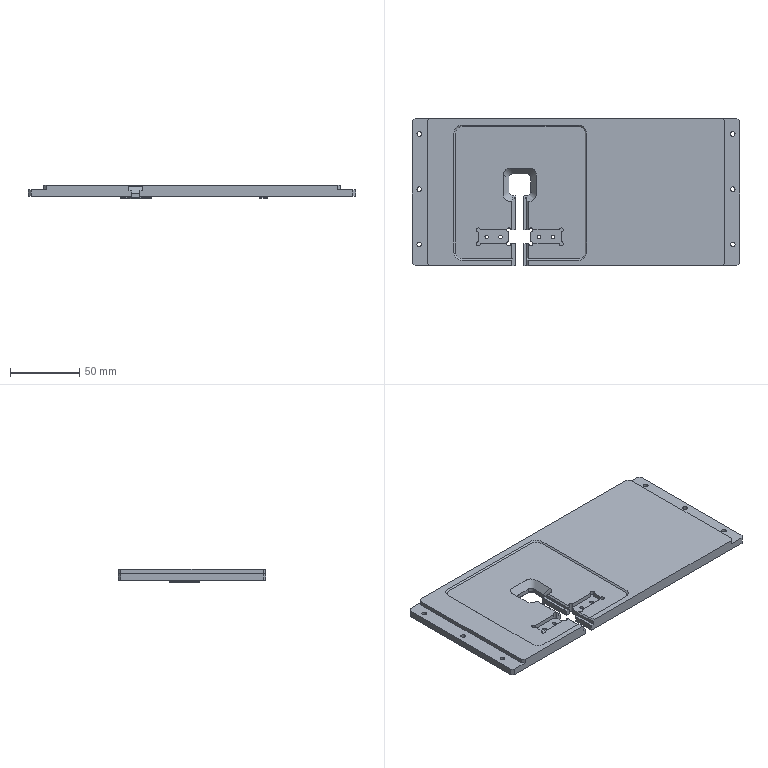NC program | NX | posted with a generic post | part box 237 x 107 x 9.5 mm
Lines 3551 to 4908 of 4908:
(FLOOR_WALL_1_1_COPY , TOOL : D10JING)
N7088 T11 M6
N7090 G54
N7092 G17 G0 G90 X119.437 Y-59. S7000 M3
N7094 G43 Z30. H11
N7096 Z-0.5
N7098 G94 G1 Z-1.5 F1000.
N7100 G3 X118.571 Y-58.5 R1.
N7102 G1 X-118.571
N7104 X-123.48 Y-53.591
N7106 X123.48
N7108 X123.5 Y-53.571
N7110 Y-48.682
N7112 X-123.5
N7114 Y-43.773
N7116 X123.5
N7118 Y-38.864
N7120 X-123.5
N7122 Y-33.955
N7124 X123.5
N7126 Y-29.045
N7128 X-123.5
N7130 Y-24.136
N7132 X123.5
N7134 Y-19.227
N7136 X-26.578
N7138 G3 X-24.231 Y-14.318 R8.5
N7140 G1 X44.986
N7142 G2 X43.061 Y-9.409 R7.5
N7144 G1 X-24.17
N7146 Y-4.5
N7148 X43.06
N7150 Y-1.3
N7152 G2 X43.257 Y0.409 R7.5
N7154 G1 X-24.17
N7156 Y2.7
N7158 G3 X-24.583 Y5.318 R8.5
N7160 G1 X47.032
N7162 Z-0.5
N7164 G0 Z30.
N7166 X44.986 Y-14.318
N7168 Z-0.5
N7170 G1 Z-1.5
N7172 G3 X50.56 Y-16.8 R7.5
N7174 G1 X52.56
N7176 G3 X58.134 Y-14.318 R7.5
N7178 G1 X123.5
N7180 Y-9.409
N7182 X60.059
N7184 X60.06 Y-9.3
N7186 Y-4.5
N7188 X123.5
N7190 Y0.409
N7192 X59.863
N7194 G3 X56.088 Y5.318 R7.5
N7196 G1 X123.5
N7198 Y10.227
N7200 X-28.722
N7202 G3 X-27.722 Y10.268 R1.
N7204 G1 Z-0.5
N7206 G0 Z30.
N7208 X-26.578 Y-19.227
N7210 Z-0.5
N7212 G1 Z-1.5
N7214 G2 X-32.67 Y-21.8 R8.5
N7216 G1 X-48.67
N7218 G2 X-54.762 Y-19.227 R8.5
N7220 G1 X-123.5
N7222 Y-14.318
N7224 X-57.109
N7226 G2 X-57.17 Y-13.3 R8.5
N7228 G1 Y-9.409
N7230 X-123.5
N7232 Y-4.5
N7234 X-57.17
N7236 Y0.409
N7238 X-123.5
N7240 Y5.318
N7242 X-56.757
N7244 G2 X-52.618 Y10.227 R8.5
N7246 G1 X-123.5
N7248 Y15.136
N7250 X123.5
N7252 Y20.045
N7254 X-123.5
N7256 Y24.955
N7258 X123.5
N7260 Y29.864
N7262 X-123.5
N7264 Y34.773
N7266 X123.5
N7268 Y39.682
N7270 X-123.5
N7272 Y44.591
N7274 X123.5
N7276 Y49.5
N7278 X-123.5
N7280 G3 X-124.366 Y49. R1.
N7282 G1 Z-0.5
N7284 G0 Z30.
N7286 X-57.67 Y-6.455
N7288 Z-0.5
N7290 G1 Z-1.5
N7292 X-57.17 Y-6.166
N7294 G3 X-56.67 Y-5.3 R1.
N7296 G1 Y2.7
N7298 G2 X-48.67 Y10.7 R8.
N7300 G1 X-32.67
N7302 G2 X-24.67 Y2.7 R8.
N7304 G1 Y-13.3
N7306 G2 X-32.67 Y-21.3 R8.
N7308 G1 X-48.67
N7310 G2 X-56.67 Y-13.3 R8.
N7312 G1 Y-5.3
N7314 G3 X-57.17 Y-4.434 R1.
N7316 G1 X-57.67 Y-4.145
N7318 Z-0.5
N7320 G0 Z30.
N7322 X42.56 Y-6.455
N7324 Z-0.5
N7326 G1 Z-1.5
N7328 X43.06 Y-6.166
N7330 G3 X43.56 Y-5.3 R1.
N7332 G1 Y-1.3
N7334 G2 X50.56 Y5.7 R7.
N7336 G1 X52.56
N7338 G2 X59.56 Y-1.3 R7.
N7340 G1 Y-9.3
N7342 G2 X52.56 Y-16.3 R7.
N7344 G1 X50.56
N7346 G2 X43.56 Y-9.3 R7.
N7348 G1 Y-5.3
N7350 G3 X43.06 Y-4.434 R1.
N7352 G1 X42.56 Y-4.145
N7354 Z-0.5
N7356 G0 Z30.
N7358 X40.004 Y-11.299
N7360 Z-6.
N7362 G1 Z-7.
N7364 G3 X40.87 Y-11.799 R1.
N7366 G1 X-11.13
N7368 Y-7.466
N7370 X40.87
N7372 Y-3.133
N7374 X-11.13
N7376 Y1.2
N7378 X40.87
N7380 Y0.334
N7382 G3 X41.37 Y1.2 R1.
N7384 G1 Y1.7
N7386 X-11.63
N7388 Y-12.3
N7390 X41.37
N7392 Y1.2
N7394 G3 X41.12 Y1.633 R0.5
N7396 G1 X40.87 Y1.2
N7398 Z-6.
N7400 G0 Z30.
N7402 M5
(ZLEVEL_PROFILE_1_COPY_COPY_1_COPY_1 , TOOL : D6R0.5)
N7404 T23 M6
N7406 G54
N7408 G17 G0 G90 X-31.962 Y-19.774 S7500 M3
N7410 G43 Z30. H23
N7412 Z0.95
N7414 G94 G1 Z-0.05 F2200.
N7416 X-32.079 Y-19.108
N7418 G3 X-32.67 Y-18.612 R0.6
N7420 G1 X-48.67
N7422 G2 X-53.982 Y-13.3 R5.312
N7424 G1 Y2.7
N7426 G2 X-48.67 Y8.012 R5.312
N7428 G1 X-44.014
N7430 G2 X-41.358 Y5.356 R2.657
N7432 G1 Y3.2
N7434 G2 X-44.17 Y0.388 R2.812
N7436 G1 X-45.67
N7438 G3 X-46.358 Y-0.3 R0.688
N7440 G1 Y-10.3
N7442 G3 X-45.67 Y-10.988 R0.688
N7444 G1 X-35.67
N7446 G3 X-34.982 Y-10.3 R0.688
N7448 G1 Y-0.3
N7450 G3 X-35.67 Y0.388 R0.688
N7452 G1 X-37.17
N7454 G2 X-39.982 Y3.2 R2.812
N7456 G1 Y5.356
N7458 G2 X-37.326 Y8.012 R2.656
N7460 G1 X-32.67
N7462 G2 X-27.358 Y2.7 R5.312
N7464 G1 Y-13.3
N7466 G2 X-32.67 Y-18.612 R5.312
N7468 G1 Y-18.679 Z-0.075
N7470 Y-18.731 Z-0.099
N7472 G3 X-27.239 Y-13.3 R5.431
N7474 G1 Y2.7
N7476 G3 X-32.67 Y8.131 R5.431
N7478 G1 X-37.384
N7480 G3 X-40.101 Y5.411 R2.718
N7482 G1 Y3.2
N7484 G3 X-37.17 Y0.269 R2.931
N7486 G1 X-35.67
N7488 G2 X-35.101 Y-0.3 R0.569
N7490 G1 Y-10.3
N7492 G2 X-35.67 Y-10.869 R0.569
N7494 G1 X-45.67
N7496 G2 X-46.239 Y-10.3 R0.569
N7498 G1 Y-0.3
N7500 G2 X-45.67 Y0.269 R0.569
N7502 G1 X-44.17
N7504 G3 X-41.239 Y3.2 R2.931
N7506 G1 Y5.412
N7508 G3 X-43.956 Y8.131 R2.718
N7510 G1 X-48.67
N7512 G3 X-54.101 Y2.7 R5.431
N7514 G1 Y-13.3
N7516 G3 X-48.67 Y-18.731 R5.431
N7518 G1 X-32.67
N7520 Y-18.773 Z-0.119
N7522 X-48.67
N7524 G2 X-54.143 Y-13.3 R5.473
N7526 G1 Y2.7
N7528 G2 X-48.67 Y8.173 R5.473
N7530 G1 X-43.934
N7532 G2 X-41.197 Y5.436 R2.737
N7534 G1 Y3.2
N7536 G2 X-44.17 Y0.227 R2.973
N7538 G1 X-45.67
N7540 G3 X-46.197 Y-0.3 R0.527
N7542 G1 Y-10.3
N7544 G3 X-45.67 Y-10.827 R0.527
N7546 G1 X-35.67
N7548 G3 X-35.143 Y-10.3 R0.527
N7550 G1 Y-0.3
N7552 G3 X-35.67 Y0.227 R0.527
N7554 G1 X-37.17
N7556 G2 X-40.143 Y3.2 R2.973
N7558 G1 Y5.435
N7560 G2 X-37.405 Y8.173 R2.738
N7562 G1 X-32.67
N7564 G2 X-27.197 Y2.7 R5.473
N7566 G1 Y-13.3
N7568 G2 X-32.67 Y-18.773 R5.473
N7570 G1 Y-18.812 Z-0.141
N7572 G3 X-27.158 Y-13.3 R5.512
N7574 G1 Y2.7
N7576 G3 X-32.67 Y8.212 R5.512
N7578 G1 X-37.424
N7580 G3 X-40.182 Y5.454 R2.758
N7582 G1 Y3.2
N7584 G3 X-37.17 Y0.188 R3.012
N7586 G1 X-35.67
N7588 G2 X-35.182 Y-0.3 R0.488
N7590 G1 Y-10.3
N7592 G2 X-35.67 Y-10.788 R0.488
N7594 G1 X-45.67
N7596 G2 X-46.158 Y-10.3 R0.488
N7598 G1 Y-0.3
N7600 G2 X-45.67 Y0.188 R0.488
N7602 G1 X-44.17
N7604 G3 X-41.158 Y3.2 R3.012
N7606 G1 Y5.456
N7608 G3 X-43.914 Y8.212 R2.756
N7610 G1 X-48.67
N7612 G3 X-54.182 Y2.7 R5.512
N7614 G1 Y-13.3
N7616 G3 X-48.67 Y-18.812 R5.512
N7618 G1 X-32.67
N7620 Y-18.85 Z-0.165
N7622 X-48.67
N7624 G2 X-54.22 Y-13.3 R5.55
N7626 G1 Y2.7
N7628 G2 X-48.67 Y8.25 R5.55
N7630 G1 X-43.897
N7632 G2 X-41.12 Y5.473 R2.776
N7634 G1 Y3.2
N7636 G2 X-44.17 Y0.15 R3.05
N7638 G1 X-45.67
N7640 G3 X-46.12 Y-0.3 R0.45
N7642 G1 Y-10.3
N7644 G3 X-45.67 Y-10.75 R0.45
N7646 G1 X-35.67
N7648 G3 X-35.22 Y-10.3 R0.45
N7650 G1 Y-0.3
N7652 G3 X-35.67 Y0.15 R0.45
N7654 G1 X-37.17
N7656 G2 X-40.22 Y3.2 R3.05
N7658 G1 Y5.472
N7660 G2 X-37.444 Y8.25 R2.777
N7662 G1 X-32.67
N7664 G2 X-27.12 Y2.7 R5.55
N7666 G1 Y-13.3
N7668 G2 X-32.67 Y-18.85 R5.55
N7670 G1 Y-18.886 Z-0.19
N7672 G3 X-27.084 Y-13.3 R5.586
N7674 G1 Y2.7
N7676 G3 X-32.67 Y8.286 R5.586
N7678 G1 X-37.462
N7680 G3 X-40.256 Y5.492 R2.794
N7682 G1 Y3.2
N7684 G3 X-37.17 Y0.114 R3.086
N7686 G1 X-35.67
N7688 G2 X-35.256 Y-0.3 R0.414
N7690 G1 Y-10.3
N7692 G2 X-35.67 Y-10.714 R0.414
N7694 G1 X-45.67
N7696 G2 X-46.084 Y-10.3 R0.414
N7698 G1 Y-0.3
N7700 G2 X-45.67 Y0.114 R0.414
N7702 G1 X-44.17
N7704 G3 X-41.084 Y3.2 R3.086
N7706 G1 Y5.492
N7708 G3 X-43.878 Y8.286 R2.794
N7710 G1 X-48.67
N7712 G3 X-54.256 Y2.7 R5.586
N7714 G1 Y-13.3
N7716 G3 X-48.67 Y-18.886 R5.586
N7718 G1 X-32.67
N7720 Y-18.922 Z-0.217
N7722 X-48.67
N7724 G2 X-54.292 Y-13.3 R5.622
N7726 G1 Y2.7
N7728 G2 X-48.67 Y8.322 R5.622
N7730 G1 X-43.86
N7732 G2 X-41.048 Y5.51 R2.812
N7734 G1 Y3.2
N7736 G2 X-44.17 Y0.078 R3.122
N7738 G1 X-45.67
N7740 G3 X-46.048 Y-0.3 R0.378
N7742 G1 Y-10.3
N7744 G3 X-45.67 Y-10.678 R0.378
N7746 G1 X-35.67
N7748 G3 X-35.292 Y-10.3 R0.378
N7750 G1 Y-0.3
N7752 G3 X-35.67 Y0.078 R0.378
N7754 G1 X-37.17
N7756 G2 X-40.292 Y3.2 R3.122
N7758 G1 Y5.51
N7760 G2 X-37.48 Y8.322 R2.812
N7762 G1 X-32.67
N7764 G2 X-27.048 Y2.7 R5.622
N7766 G1 Y-13.3
N7768 G2 X-32.67 Y-18.922 R5.622
N7770 G1 Y-18.957 Z-0.246
N7772 G3 X-27.013 Y-13.3 R5.657
N7774 G1 Y2.7
N7776 G3 X-32.67 Y8.357 R5.657
N7778 G1 X-37.498
N7780 G3 X-40.327 Y5.527 R2.829
N7782 G1 Y3.2
N7784 G3 X-37.17 Y0.043 R3.157
N7786 G1 X-35.67
N7788 G2 X-35.327 Y-0.3 R0.343
N7790 G1 Y-10.3
N7792 G2 X-35.67 Y-10.643 R0.343
N7794 G1 X-45.67
N7796 G2 X-46.013 Y-10.3 R0.343
N7798 G1 Y-0.3
N7800 G2 X-45.67 Y0.043 R0.343
N7802 G1 X-44.17
N7804 G3 X-41.013 Y3.2 R3.157
N7806 G1 Y5.528
N7808 G3 X-43.842 Y8.357 R2.829
N7810 G1 X-48.67
N7812 G3 X-54.327 Y2.7 R5.657
N7814 G1 Y-13.3
N7816 G3 X-48.67 Y-18.957 R5.657
N7818 G1 X-32.67
N7820 Y-18.99 Z-0.276
N7822 X-48.67
N7824 G2 X-54.36 Y-13.3 R5.69
N7826 G1 Y2.7
N7828 G2 X-48.67 Y8.39 R5.69
N7830 G1 X-43.825
N7832 G2 X-40.98 Y5.544 R2.846
N7834 G1 Y3.2
N7836 G2 X-44.17 Y0.01 R3.19
N7838 G1 X-45.67
N7840 G3 X-45.98 Y-0.3 R0.31
N7842 G1 Y-10.3
N7844 G3 X-45.67 Y-10.61 R0.31
N7846 G1 X-35.67
N7848 G3 X-35.36 Y-10.3 R0.31
N7850 G1 Y-0.3
N7852 G3 X-35.67 Y0.01 R0.31
N7854 G1 X-37.17
N7856 G2 X-40.36 Y3.2 R3.19
N7858 G1 Y5.543
N7860 G2 X-37.515 Y8.39 R2.846
N7862 G1 X-32.67
N7864 G2 X-26.98 Y2.7 R5.69
N7866 G1 Y-13.3
N7868 G2 X-32.67 Y-18.99 R5.69
N7870 G1 Y-19.023 Z-0.309
N7872 G3 X-26.947 Y-13.3 R5.723
N7874 G1 Y2.7
N7876 G3 X-32.67 Y8.423 R5.723
N7878 G1 X-37.531
N7880 G3 X-40.393 Y5.561 R2.862
N7882 G1 Y3.2
N7884 G3 X-37.17 Y-0.023 R3.223
N7886 G1 X-35.67
N7888 G2 X-35.393 Y-0.3 R0.277
N7890 G1 Y-10.3
N7892 G2 X-35.67 Y-10.577 R0.277
N7894 G1 X-45.67
N7896 G2 X-45.947 Y-10.3 R0.277
N7898 G1 Y-0.3
N7900 G2 X-45.67 Y-0.023 R0.277
N7902 G1 X-44.17
N7904 G3 X-40.947 Y3.2 R3.223
N7906 G1 Y5.561
N7908 G3 X-43.809 Y8.423 R2.861
N7910 G1 X-48.67
N7912 G3 X-54.393 Y2.7 R5.723
N7914 G1 Y-13.3
N7916 G3 X-48.67 Y-19.023 R5.723
N7918 G1 X-32.67
N7920 Y-19.054 Z-0.343
N7922 X-48.67
N7924 G2 X-54.424 Y-13.3 R5.754
N7926 G1 Y2.7
N7928 G2 X-48.67 Y8.454 R5.754
N7930 G1 X-43.794
N7932 G2 X-40.916 Y5.577 R2.877
N7934 G1 Y3.2
N7936 G2 X-44.17 Y-0.054 R3.254
N7938 G1 X-45.67
N7940 G3 X-45.916 Y-0.3 R0.246
N7942 G1 Y-10.3
N7944 G3 X-45.67 Y-10.546 R0.246
N7946 G1 X-35.67
N7948 G3 X-35.424 Y-10.3 R0.246
N7950 G1 Y-0.3
N7952 G3 X-35.67 Y-0.054 R0.246
N7954 G1 X-37.17
N7956 G2 X-40.424 Y3.2 R3.254
N7958 G1 Y5.577
N7960 G2 X-37.547 Y8.454 R2.877
N7962 G1 X-32.67
N7964 G2 X-26.916 Y2.7 R5.754
N7966 G1 Y-13.3
N7968 G2 X-32.67 Y-19.054 R5.754
N7970 G1 Y-19.084 Z-0.379
N7972 G3 X-26.886 Y-13.3 R5.784
N7974 G1 Y2.7
N7976 G3 X-32.67 Y8.484 R5.784
N7978 G1 X-37.562
N7980 G3 X-40.454 Y5.591 R2.892
N7982 G1 Y3.2
N7984 G3 X-37.17 Y-0.084 R3.284
N7986 G1 X-35.67
N7988 G2 X-35.454 Y-0.3 R0.216
N7990 G1 Y-10.3
N7992 G2 X-35.67 Y-10.516 R0.216
N7994 G1 X-45.67
N7996 G2 X-45.886 Y-10.3 R0.216
N7998 G1 Y-0.3
N8000 G2 X-45.67 Y-0.084 R0.216
N8002 G1 X-44.17
N8004 G3 X-40.886 Y3.2 R3.284
N8006 G1 Y5.592
N8008 G3 X-43.779 Y8.484 R2.892
N8010 G1 X-48.67
N8012 G3 X-54.454 Y2.7 R5.784
N8014 G1 Y-13.3
N8016 G3 X-48.67 Y-19.084 R5.784
N8018 G1 X-32.67
N8020 Y-19.112 Z-0.416
N8022 X-48.67
N8024 G2 X-54.482 Y-13.3 R5.812
N8026 G1 Y2.7
N8028 G2 X-48.67 Y8.512 R5.812
N8030 G1 X-43.765
N8032 G2 X-40.858 Y5.606 R2.906
N8034 G1 Y3.2
N8036 G2 X-44.17 Y-0.112 R3.312
N8038 G1 X-45.67
N8040 G3 X-45.858 Y-0.3 R0.188
N8042 G1 Y-10.3
N8044 G3 X-45.67 Y-10.488 R0.188
N8046 G1 X-35.67
N8048 G3 X-35.482 Y-10.3 R0.188
N8050 G1 Y-0.3
N8052 G3 X-35.67 Y-0.112 R0.188
N8054 G1 X-37.17
N8056 G2 X-40.482 Y3.2 R3.312
N8058 G1 Y5.605
N8060 G2 X-37.576 Y8.512 R2.906
N8062 G1 X-32.67
N8064 G2 X-26.858 Y2.7 R5.812
N8066 G1 Y-13.3
N8068 G2 X-32.67 Y-19.112 R5.812
N8070 G1 Y-19.139 Z-0.455
N8072 G3 X-26.831 Y-13.3 R5.839
N8074 G1 Y2.7
N8076 G3 X-32.67 Y8.539 R5.839
N8078 G1 X-37.589
N8080 G3 X-40.509 Y5.619 R2.92
N8082 G1 Y3.2
N8084 G3 X-37.17 Y-0.139 R3.339
N8086 G1 X-35.67
N8088 G2 X-35.509 Y-0.3 R0.161
N8090 G1 Y-10.3
N8092 G2 X-35.67 Y-10.461 R0.161
N8094 G1 X-45.67
N8096 G2 X-45.831 Y-10.3 R0.161
N8098 G1 Y-0.3
N8100 G2 X-45.67 Y-0.139 R0.161
N8102 G1 X-44.17
N8104 G3 X-40.831 Y3.2 R3.339
N8106 G1 Y5.619
N8108 G3 X-43.751 Y8.539 R2.92
N8110 G1 X-48.67
N8112 G3 X-54.509 Y2.7 R5.839
N8114 G1 Y-13.3
N8116 G3 X-48.67 Y-19.139 R5.839
N8118 G1 X-32.67
N8120 Y-19.164 Z-0.496
N8122 X-48.67
N8124 G2 X-54.534 Y-13.3 R5.864
N8126 G1 Y2.7
N8128 G2 X-48.67 Y8.564 R5.864
N8130 G1 X-43.739
N8132 G2 X-40.806 Y5.631 R2.934
N8134 G1 Y3.2
N8136 G2 X-44.17 Y-0.164 R3.364
N8138 G1 X-45.67
N8140 G3 X-45.806 Y-0.3 R0.136
N8142 G1 Y-10.3
N8144 G3 X-45.67 Y-10.436 R0.136
N8146 G1 X-35.67
N8148 G3 X-35.534 Y-10.3 R0.136
N8150 G1 Y-0.3
N8152 G3 X-35.67 Y-0.164 R0.136
N8154 G1 X-37.17
N8156 G2 X-40.534 Y3.2 R3.364
N8158 G1 Y5.631
N8160 G2 X-37.601 Y8.564 R2.933
N8162 G1 X-32.67
N8164 G2 X-26.806 Y2.7 R5.864
N8166 G1 Y-13.3
N8168 G2 X-32.67 Y-19.164 R5.864
N8170 G3 X-33.261 Y-19.659 R0.6
N8172 G1 X-33.385 Y-20.364
N8174 Z0.504
N8176 G0 Z30.
N8178 X-42.647 Y8.381
N8180 Z0.504
N8182 G1 Z-0.537
N8184 G3 X-43.727 Y8.586 R3.202
N8186 G1 X-48.67
N8188 G3 X-54.556 Y2.7 R5.886
N8190 G1 Y-13.3
N8192 G3 X-48.67 Y-19.186 R5.886
N8194 G1 X-32.67
N8196 G3 X-26.784 Y-13.3 R5.886
N8198 G1 Y2.7
N8200 G3 X-32.67 Y8.586 R5.886
N8202 G1 X-37.614
N8204 G3 X-38.394 Y8.477 R2.844
N8206 G1 X-38.426 Y8.468
N8208 X-38.868 Y8.382
N8210 X-38.869 Y8.425 Z-0.558
N8212 Y8.461 Z-0.579
N8214 G3 X-38.423 Y8.499 R1.403
N8216 G2 X-37.622 Y8.607 R3.693
N8218 G1 X-32.67
N8220 G2 X-26.763 Y2.7 R5.907
N8222 G1 Y-13.3
N8224 G2 X-32.67 Y-19.207 R5.907
N8226 G1 X-48.67
N8228 G2 X-54.577 Y-13.3 R5.907
N8230 G1 Y2.7
N8232 G2 X-48.67 Y8.607 R5.907
N8234 G1 X-43.718
N8236 G2 X-42.812 Y8.466 R3.128
N8238 G1 X-42.929 Y8.525 Z-0.622
N8240 G3 X-43.707 Y8.626 R3.577
N8242 G1 X-48.67
N8244 G3 X-54.596 Y2.7 R5.926
N8246 G1 Y-13.3
N8248 G3 X-48.67 Y-19.226 R5.926
N8250 G1 X-32.67
N8252 G3 X-26.744 Y-13.3 R5.926
N8254 G1 Y2.7
N8256 G3 X-32.67 Y8.626 R5.926
N8258 G1 X-37.632
N8260 G3 X-38.426 Y8.525 R4.19
N8262 G1 X-38.869 Y8.522
N8264 X-38.87 Y8.552 Z-0.645
N8266 Y8.565 Z-0.667
N8268 X-38.326 Y8.57
N8270 G2 X-37.64 Y8.643 R4.259
N8272 G1 X-32.67
N8274 G2 X-26.727 Y2.7 R5.943
N8276 G1 Y-13.3
N8278 G2 X-32.67 Y-19.243 R5.943
N8280 G1 X-48.67
N8282 G2 X-54.613 Y-13.3 R5.943
N8284 G1 Y2.7
N8286 G2 X-48.67 Y8.643 R5.943
N8288 G1 X-43.699
N8290 G2 X-43.002 Y8.571 R5.372
N8292 G1 X-42.955 Y8.607 Z-0.713
N8294 X-43.03 Y8.609
N8296 X-43.692 Y8.658
N8298 X-48.67
N8300 G3 X-54.628 Y2.7 R5.958
N8302 G1 Y-13.3
N8304 G3 X-48.67 Y-19.258 R5.958
N8306 G1 X-32.67
N8308 G3 X-26.712 Y-13.3 R5.958
N8310 G1 Y2.7
N8312 G3 X-32.67 Y8.658 R5.958
N8314 G1 X-37.648
N8316 X-37.735 Y8.656
N8318 X-38.244 Y8.608
N8320 X-38.869 Y8.605
N8322 Y8.634 Z-0.759
N8324 G3 X-37.655 Y8.671 R11.466
N8326 G1 X-32.67
N8328 G2 X-26.699 Y2.7 R5.971
N8330 G1 Y-13.3
N8332 G2 X-32.67 Y-19.271 R5.971
N8334 G1 X-48.67
N8336 G2 X-54.641 Y-13.3 R5.971
N8338 G1 Y2.7
N8340 G2 X-48.67 Y8.671 R5.971
N8342 G1 X-43.686
N8344 G3 X-42.869 Y8.636 R6.276
N8346 G1 X-42.795 Y8.659 Z-0.807
N8348 G2 X-43.68 Y8.681 R9.251
N8350 G1 X-48.67
N8352 G3 X-54.651 Y2.7 R5.981
N8354 G1 Y-13.3
N8356 G3 X-48.67 Y-19.281 R5.981
N8358 G1 X-32.67
N8360 G3 X-26.689 Y-13.3 R5.981
N8362 G1 Y2.7
N8364 G3 X-32.67 Y8.681 R5.981
N8366 G1 X-37.661
N8368 X-38.25 Y8.654
N8370 X-38.336
N8372 X-38.426 Y8.657
N8374 X-38.868 Y8.655
N8376 Y8.669 Z-0.831
N8378 Y8.672 Z-0.855
N8380 G3 X-37.664 Y8.689 R40.619
N8382 G1 X-32.67
N8384 G2 X-26.681 Y2.7 R5.989
N8386 G1 Y-13.3
N8388 G2 X-32.67 Y-19.289 R5.989
N8390 G1 X-48.67
N8392 G2 X-54.659 Y-13.3 R5.989
N8394 G1 Y2.7
N8396 G2 X-48.67 Y8.689 R5.989
N8398 G1 X-43.676
N8400 G3 X-42.723 Y8.675 R22.668
N8402 G1 X-42.67 Y8.689 Z-0.903
N8404 X-43.605 Y8.692
N8406 X-43.673 Y8.695
N8408 X-48.67
N8410 G3 X-54.665 Y2.7 R5.995
N8412 G1 Y-13.3
N8414 G3 X-48.67 Y-19.295 R5.995
N8416 G1 X-32.67
N8418 G3 X-26.675 Y-13.3 R5.995
N8420 G1 Y2.7
N8422 G3 X-32.67 Y8.695 R5.995
N8424 G1 X-37.667
N8426 X-37.735 Y8.693
N8428 X-38.863 Y8.688
N8430 X-38.856 Y8.695 Z-0.952
N8432 X-38.771 Y8.698
N8434 X-37.735
N8436 X-37.669 Y8.699
N8438 X-32.67
N8440 G2 X-26.671 Y2.7 R5.999
N8442 G1 Y-13.3
N8444 G2 X-32.67 Y-19.299 R5.999
N8446 G1 X-48.67
N8448 G2 X-54.669 Y-13.3 R5.999
N8450 G1 Y2.7
N8452 G2 X-48.67 Y8.699 R5.999
N8454 G1 X-43.671
N8456 X-43.605 Y8.697
N8458 X-42.585 Y8.698
N8460 X-42.569 Y8.7 Z-1.
N8462 X-43.671
N8464 X-48.67
N8466 G3 X-54.67 Y2.7 R6.
N8468 G1 Y-13.3
N8470 G3 X-48.67 Y-19.3 R6.
N8472 G1 X-32.67
N8474 G3 X-26.67 Y-13.3 R6.
N8476 G1 Y2.7
N8478 G3 X-32.67 Y8.7 R6.
N8480 G1 X-37.735
N8482 X-38.771
N8484 X-38.849 Y8.698
N8486 G2 X-39.454 Y9.176 R0.6
N8488 G1 X-39.59 Y9.837
N8490 Z0.
N8492 G0 Z30.
N8494 X-44.584 Y-9.214
N8496 Z0.463
N8498 G1 Z-0.537
N8500 X-45.174 Y-9.823
N8502 G3 X-45.67 Y-10.414 R0.6
N8504 G1 X-35.67
N8506 X-35.608 Y-10.407
N8508 X-35.563 Y-10.362
N8510 X-35.556 Y-10.3
N8512 Y-0.3
N8514 X-35.563 Y-0.238
N8516 X-35.608 Y-0.193
N8518 X-35.67 Y-0.186
N8520 X-37.17
N8522 G2 X-40.556 Y3.2 R3.386
N8524 G1 Y3.61
N8526 G3 X-40.784 Y3.615 R0.131
N8528 G1 Y3.2
N8530 G2 X-44.17 Y-0.186 R3.386
N8532 G1 X-45.67
N8534 X-45.732 Y-0.193
N8536 X-45.777 Y-0.238
N8538 X-45.784 Y-0.3
N8540 Y-10.3
N8542 X-45.777 Y-10.362
N8544 X-45.732 Y-10.407
N8546 X-45.67 Y-10.414
N8548 Y-10.393 Z-0.579
N8550 X-45.722 Y-10.389
N8552 X-45.759 Y-10.352
N8554 X-45.763 Y-10.3
N8556 Y-0.3
N8558 X-45.759 Y-0.248
N8560 X-45.722 Y-0.211
N8562 X-45.67 Y-0.207
N8564 X-44.17
N8566 G3 X-40.763 Y3.2 R3.407
N8568 G1 Y3.524
N8570 G2 X-40.577 Y3.523 R0.096
N8572 G1 Y3.2
N8574 G3 X-37.17 Y-0.207 R3.407
N8576 G1 X-35.67
N8578 X-35.618 Y-0.211
N8580 X-35.581 Y-0.248
N8582 X-35.577 Y-0.3
N8584 Y-10.3
N8586 X-35.581 Y-10.352
N8588 X-35.618 Y-10.389
N8590 X-35.67 Y-10.393
N8592 X-45.67
N8594 Y-10.374 Z-0.622
N8596 X-35.67
N8598 X-35.628 Y-10.373
N8600 X-35.597 Y-10.342
N8602 X-35.596 Y-10.3
N8604 Y-0.3
N8606 X-35.597 Y-0.258
N8608 X-35.628 Y-0.227
N8610 X-35.67 Y-0.226
N8612 X-37.17
N8614 G2 X-40.596 Y3.2 R3.426
N8616 G1 Y3.462
N8618 X-40.636 Y3.515
N8620 X-40.705 Y3.514
N8622 X-40.744 Y3.461
N8624 Y3.2
N8626 G2 X-44.17 Y-0.226 R3.426
N8628 G1 X-45.67
N8630 X-45.712 Y-0.227
N8632 X-45.743 Y-0.258
N8634 X-45.744 Y-0.3
N8636 Y-10.3
N8638 X-45.743 Y-10.342
N8640 X-45.712 Y-10.373
N8642 X-45.67 Y-10.374
N8644 Y-10.357 Z-0.667
N8646 X-45.704 Y-10.358
N8648 X-45.728 Y-10.334
N8650 X-45.727 Y-10.3
N8652 Y-0.3
N8654 X-45.728 Y-0.266
N8656 X-45.704 Y-0.242
N8658 X-45.67 Y-0.243
N8660 X-44.17
N8662 G3 X-40.727 Y3.2 R3.443
N8664 G1 Y3.418
N8666 X-40.697 Y3.458
N8668 X-40.644
N8670 X-40.613 Y3.419
N8672 Y3.2
N8674 G3 X-37.17 Y-0.243 R3.443
N8676 G1 X-35.67
N8678 X-35.636 Y-0.242
N8680 X-35.612 Y-0.266
N8682 X-35.613 Y-0.3
N8684 Y-10.3
N8686 X-35.612 Y-10.334
N8688 X-35.636 Y-10.358
N8690 X-35.67 Y-10.357
N8692 X-45.67
N8694 Y-10.342 Z-0.713
N8696 X-35.67
N8698 X-35.644 Y-10.345
N8700 X-35.625 Y-10.326
N8702 X-35.628 Y-10.3
N8704 Y-0.3
N8706 X-35.625 Y-0.274
N8708 X-35.644 Y-0.255
N8710 X-35.67 Y-0.258
N8712 X-37.17
N8714 G2 X-40.628 Y3.2 R3.458
N8716 G1 Y3.385
N8718 X-40.65 Y3.415
N8720 X-40.69
N8722 X-40.712 Y3.385
N8724 Y3.2
N8726 G2 X-44.17 Y-0.258 R3.458
N8728 G1 X-45.67
N8730 X-45.696 Y-0.255
N8732 X-45.715 Y-0.274
N8734 X-45.712 Y-0.3
N8736 Y-10.3
N8738 X-45.715 Y-10.326
N8740 X-45.696 Y-10.345
N8742 X-45.67 Y-10.342
N8744 Y-10.329 Z-0.759
N8746 X-45.69 Y-10.334
N8748 X-45.704 Y-10.32
N8750 X-45.699 Y-10.3
N8752 Y-0.3
N8754 X-45.704 Y-0.28
N8756 X-45.69 Y-0.266
N8758 X-45.67 Y-0.271
N8760 X-44.17
N8762 G3 X-40.699 Y3.2 R3.471
N8764 G1 Y3.356
N8766 X-40.685 Y3.38
N8768 X-40.656
N8770 X-40.641 Y3.357
N8772 Y3.2
N8774 G3 X-37.17 Y-0.271 R3.471
N8776 G1 X-35.67
N8778 X-35.65 Y-0.266
N8780 X-35.636 Y-0.28
N8782 X-35.641 Y-0.3
N8784 Y-10.3
N8786 X-35.636 Y-10.32
N8788 X-35.65 Y-10.334
N8790 X-35.67 Y-10.329
N8792 X-45.67
N8794 Y-10.319 Z-0.807
N8796 X-35.67
N8798 X-35.65 Y-10.32
N8800 X-35.651 Y-10.3
N8802 Y-0.3
N8804 X-35.65 Y-0.28
N8806 X-35.67 Y-0.281
N8808 X-37.17
N8810 G2 X-40.651 Y3.2 R3.481
N8812 G1 Y3.336
N8814 X-40.66 Y3.354
N8816 X-40.68
N8818 X-40.689 Y3.336
N8820 Y3.2
N8822 G2 X-44.17 Y-0.281 R3.481
N8824 G1 X-45.67
N8826 X-45.69 Y-0.28
N8828 X-45.689 Y-0.3
N8830 Y-10.3
N8832 X-45.69 Y-10.32
N8834 X-45.67 Y-10.319
N8836 Y-10.311 Z-0.855
N8838 X-45.681
N8840 Y-10.3
N8842 Y-0.3
N8844 Y-0.289
N8846 X-45.67
N8848 X-44.17
N8850 G3 X-40.681 Y3.2 R3.489
N8852 G1 Y3.32
N8854 X-40.659
N8856 Y3.2
N8858 G3 X-37.17 Y-0.289 R3.489
N8860 G1 X-35.67
N8862 X-35.659
N8864 Y-0.3
N8866 Y-10.3
N8868 Y-10.311
N8870 X-35.67
N8872 X-45.67
N8874 Y-10.305 Z-0.903
N8876 X-35.67
N8878 X-35.665
N8880 Y-10.3
N8882 Y-0.3
N8884 Y-0.295
N8886 X-35.67
N8888 X-37.17
N8890 G2 X-40.665 Y3.2 R3.495
N8892 G1 Y3.29
N8894 X-40.675 Y3.2
N8896 G2 X-44.17 Y-0.295 R3.495
N8898 G1 X-45.67
N8900 X-45.675
N8902 Y-0.3
N8904 Y-10.3
N8906 Y-10.305
N8908 X-45.67
N8910 G3 X-45.079 Y-9.809 R0.6
N8912 G1 X-44.475 Y-9.105
N8914 Z0.097
N8916 G0 Z30.
N8918 X-44.472 Y-9.102
N8920 Z0.048
N8922 G1 Z-0.952
N8924 X-45.079 Y-9.803
N8926 G2 X-45.67 Y-10.299 R0.6
N8928 G1 X-45.672 Y-10.134
N8930 Y-0.466
N8932 X-45.669 Y-0.299
N8934 X-44.17
N8936 G3 X-40.676 Y3.017 R3.499
N8938 G1 X-40.669 Y3.29
N8940 Y3.2
N8942 G3 X-37.325 Y-0.295 R3.499
N8944 G1 X-37.17 Y-0.299
N8946 X-35.684
N8948 X-35.669 Y-0.301
N8950 Y-10.299
N8952 X-35.836 Y-10.302
N8954 X-45.504
N8956 X-45.67 Y-10.299
N8958 Z-1.
N8960 X-45.504 Y-10.301
N8962 X-35.836
N8964 X-35.67 Y-10.299
N8966 Y-0.466
N8968 X-35.672 Y-0.303
N8970 X-35.836 Y-0.3
N8972 X-37.17
N8974 X-37.325 Y-0.297
N8976 G2 X-40.663 Y2.975 R3.5
N8978 G1 X-40.67 Y3.29
N8980 Y3.018
N8982 X-40.707 Y2.704
N8984 G2 X-40.843 Y2.115 R3.358
N8986 G1 X-40.865 Y2.051
N8988 G2 X-41.939 Y0.491 R3.614
N8990 X-42.721 Y0.014 R4.361
N8992 X-44.17 Y-0.3 R3.5
N8994 G1 X-45.504
N8996 X-45.668 Y-0.302
N8998 X-45.671 Y-0.466
N9000 Y-10.134
N9002 X-45.67 Y-10.299
N9004 G3 X-45.079 Y-9.803 R0.6
N9006 G1 X-44.471 Y-9.101
N9008 Z0.
N9010 G0 Z30.
N9012 X45.212 Y-10.007
N9014 Z0.881
N9016 G1 Z-0.119
N9018 X45.869 Y-9.891
N9020 G3 X46.365 Y-9.3 R0.6
N9022 G1 Y-1.3
N9024 G2 X50.56 Y2.895 R4.195
N9026 G1 X52.56
N9028 G2 X56.755 Y-1.3 R4.195
N9030 G1 Y-9.3
N9032 G2 X52.56 Y-13.495 R4.195
N9034 G1 X50.56
N9036 G2 X46.365 Y-9.3 R4.195
N9038 G1 X46.317 Z-0.13
N9040 X46.277 Z-0.141
N9042 G3 X50.56 Y-13.583 R4.283
N9044 G1 X52.56
N9046 G3 X56.843 Y-9.3 R4.283
N9048 G1 Y-1.3
N9050 G3 X52.56 Y2.983 R4.283
N9052 G1 X50.56
N9054 G3 X46.277 Y-1.3 R4.283
N9056 G1 Y-9.3
N9058 X46.24 Z-0.153
N9060 X46.207 Z-0.165
N9062 Y-1.3
N9064 G2 X50.56 Y3.053 R4.353
N9066 G1 X52.56
N9068 G2 X56.913 Y-1.3 R4.353
N9070 G1 Y-9.3
N9072 G2 X52.56 Y-13.653 R4.353
N9074 G1 X50.56
N9076 G2 X46.207 Y-9.3 R4.353
N9078 G1 X46.175 Z-0.177
N9080 X46.146 Z-0.19
N9082 G3 X50.56 Y-13.714 R4.414
N9084 G1 X52.56
N9086 G3 X56.974 Y-9.3 R4.414
N9088 G1 Y-1.3
N9090 G3 X52.56 Y3.114 R4.414
N9092 G1 X50.56
N9094 G3 X46.146 Y-1.3 R4.414
N9096 G1 Y-9.3
N9098 X46.091 Z-0.217
N9100 Y-1.3
N9102 G2 X50.56 Y3.169 R4.469
N9104 G1 X52.56
N9106 G2 X57.029 Y-1.3 R4.469
N9108 G1 Y-9.3
N9110 G2 X52.56 Y-13.769 R4.469
N9112 G1 X50.56
N9114 G2 X46.091 Y-9.3 R4.469
N9116 G1 X46.04 Z-0.246
N9118 G3 X50.56 Y-13.82 R4.52
N9120 G1 X52.56
N9122 G3 X57.08 Y-9.3 R4.52
N9124 G1 Y-1.3
N9126 G3 X52.56 Y3.22 R4.52
N9128 G1 X50.56
N9130 G3 X46.04 Y-1.3 R4.52
N9132 G1 Y-9.3
N9134 X45.993 Z-0.276
N9136 Y-1.3
N9138 G2 X50.56 Y3.267 R4.567
N9140 G1 X52.56
N9142 G2 X57.127 Y-1.3 R4.567
N9144 G1 Y-9.3
N9146 G2 X52.56 Y-13.867 R4.567
N9148 G1 X50.56
N9150 G2 X45.993 Y-9.3 R4.567
N9152 G1 X45.949 Z-0.309
N9154 G3 X50.56 Y-13.911 R4.611
N9156 G1 X52.56
N9158 G3 X57.171 Y-9.3 R4.611
N9160 G1 Y-1.3
N9162 G3 X52.56 Y3.311 R4.611
N9164 G1 X50.56
N9166 G3 X45.949 Y-1.3 R4.611
N9168 G1 Y-9.3
N9170 X45.907 Z-0.343
N9172 Y-1.3
N9174 G2 X50.56 Y3.353 R4.653
N9176 G1 X52.56
N9178 G2 X57.213 Y-1.3 R4.653
N9180 G1 Y-9.3
N9182 G2 X52.56 Y-13.953 R4.653
N9184 G1 X50.56
N9186 G2 X45.907 Y-9.3 R4.653
N9188 G1 X45.867 Z-0.379
N9190 G3 X50.56 Y-13.993 R4.693
N9192 G1 X52.56
N9194 G3 X57.253 Y-9.3 R4.693
N9196 G1 Y-1.3
N9198 G3 X52.56 Y3.393 R4.693
N9200 G1 X50.56
N9202 G3 X45.867 Y-1.3 R4.693
N9204 G1 Y-9.3
N9206 X45.83 Z-0.416
N9208 Y-1.3
N9210 G2 X50.56 Y3.43 R4.73
N9212 G1 X52.56
N9214 G2 X57.29 Y-1.3 R4.73
N9216 G1 Y-9.3
N9218 G2 X52.56 Y-14.03 R4.73
N9220 G1 X50.56
N9222 G2 X45.83 Y-9.3 R4.73
N9224 G1 X45.796 Z-0.455
N9226 G3 X50.56 Y-14.064 R4.764
N9228 G1 X52.56
N9230 G3 X57.324 Y-9.3 R4.764
N9232 G1 Y-1.3
N9234 G3 X52.56 Y3.464 R4.764
N9236 G1 X50.56
N9238 G3 X45.796 Y-1.3 R4.764
N9240 G1 Y-9.3
N9242 X45.763 Z-0.496
N9244 Y-1.3
N9246 G2 X50.56 Y3.497 R4.797
N9248 G1 X52.56
N9250 G2 X57.357 Y-1.3 R4.797
N9252 G1 Y-9.3
N9254 G2 X52.56 Y-14.097 R4.797
N9256 G1 X50.56
N9258 G2 X45.763 Y-9.3 R4.797
N9260 G1 X45.734 Z-0.537
N9262 G3 X50.56 Y-14.126 R4.826
N9264 G1 X52.56
N9266 G3 X57.386 Y-9.3 R4.826
N9268 G1 Y-1.3
N9270 G3 X52.56 Y3.526 R4.826
N9272 G1 X50.56
N9274 G3 X45.734 Y-1.3 R4.826
N9276 G1 Y-9.3
N9278 X45.707 Z-0.579
N9280 Y-1.3
N9282 G2 X50.56 Y3.553 R4.853
N9284 G1 X52.56
N9286 G2 X57.413 Y-1.3 R4.853
N9288 G1 Y-9.3
N9290 G2 X52.56 Y-14.153 R4.853
N9292 G1 X50.56
N9294 G2 X45.707 Y-9.3 R4.853
N9296 G1 X45.682 Z-0.622
N9298 G3 X50.56 Y-14.178 R4.878
N9300 G1 X52.56
N9302 G3 X57.438 Y-9.3 R4.878
N9304 G1 Y-1.3
N9306 G3 X52.56 Y3.578 R4.878
N9308 G1 X50.56
N9310 G3 X45.682 Y-1.3 R4.878
N9312 G1 Y-9.3
N9314 X45.659 Z-0.667
N9316 Y-1.3
N9318 G2 X50.56 Y3.601 R4.901
N9320 G1 X52.56
N9322 G2 X57.461 Y-1.3 R4.901
N9324 G1 Y-9.3
N9326 G2 X52.56 Y-14.201 R4.901
N9328 G1 X50.56
N9330 G2 X45.659 Y-9.3 R4.901
N9332 G1 X45.638 Z-0.713
N9334 G3 X50.56 Y-14.222 R4.922
N9336 G1 X52.56
N9338 G3 X57.482 Y-9.3 R4.922
N9340 G1 Y-1.3
N9342 G3 X52.56 Y3.622 R4.922
N9344 G1 X50.56
N9346 G3 X45.638 Y-1.3 R4.922
N9348 G1 Y-9.3
N9350 X45.62 Z-0.759
N9352 Y-1.3
N9354 G2 X50.56 Y3.64 R4.94
N9356 G1 X52.56
N9358 G2 X57.5 Y-1.3 R4.94
N9360 G1 Y-9.3
N9362 G2 X52.56 Y-14.24 R4.94
N9364 G1 X50.56
N9366 G2 X45.62 Y-9.3 R4.94
N9368 G1 X45.604 Z-0.807
N9370 G3 X50.56 Y-14.256 R4.956
N9372 G1 X52.56
N9374 G3 X57.516 Y-9.3 R4.956
N9376 G1 Y-1.3
N9378 G3 X52.56 Y3.656 R4.956
N9380 G1 X50.56
N9382 G3 X45.604 Y-1.3 R4.956
N9384 G1 Y-9.3
N9386 X45.591 Z-0.855
N9388 Y-1.3
N9390 G2 X50.56 Y3.669 R4.969
N9392 G1 X52.56
N9394 G2 X57.529 Y-1.3 R4.969
N9396 G1 Y-9.3
N9398 G2 X52.56 Y-14.269 R4.969
N9400 G1 X50.56
N9402 G2 X45.591 Y-9.3 R4.969
N9404 G1 X45.58 Z-0.903
N9406 G3 X50.56 Y-14.28 R4.98
N9408 G1 X52.56
N9410 G3 X57.54 Y-9.3 R4.98
N9412 G1 Y-1.3
N9414 G3 X52.56 Y3.68 R4.98
N9416 G1 X50.56
N9418 G3 X45.58 Y-1.3 R4.98
N9420 G1 Y-9.3
N9422 X45.571 Z-0.952
N9424 Y-1.3
N9426 G2 X50.56 Y3.689 R4.989
N9428 G1 X52.56
N9430 G2 X57.549 Y-1.3 R4.989
N9432 G1 Y-9.3
N9434 G2 X52.56 Y-14.289 R4.989
N9436 G1 X50.56
N9438 G2 X45.571 Y-9.3 R4.989
N9440 G1 X45.565 Z-1.
N9442 G3 X50.56 Y-14.295 R4.995
N9444 G1 X52.56
N9446 G3 X57.555 Y-9.3 R4.995
N9448 G1 Y-1.3
N9450 G3 X52.56 Y3.695 R4.995
N9452 G1 X50.56
N9454 G3 X45.565 Y-1.3 R4.995
N9456 G1 Y-9.3
N9458 G2 X45.069 Y-9.891 R0.6
N9460 G1 X44.406 Y-10.008
N9462 Z0.
N9464 G0 Z30.
N9466 M5
(ZLEVEL_PROFILE_1_COPY_1_COPY_COPY_1 , TOOL : D6A45)
N9468 T22 M6
N9470 G54
N9472 G17 G0 G90 X114.191 Y-2. S7500 M3
N9474 G43 Z30. H22
N9476 Z-0.5
N9478 G94 G1 Z-2.5 F1000.
N9480 G3 X113.5 Y-1.309 R0.691
N9482 X114.191 Y-2. R-0.691
N9484 X113.891 Y-1.48 R0.6
N9486 G1 Z-1.5
N9488 G0 Z30.
N9490 X114.191 Y-42.
N9492 Z-0.5
N9494 G1 Z-2.5
N9496 G3 X113.5 Y-41.309 R0.691
N9498 X114.191 Y-42. R-0.691
N9500 X113.891 Y-41.48 R0.6
N9502 G1 Z-1.5
N9504 G0 Z30.
N9506 X-114.191 Y-2.
N9508 Z-0.5
N9510 G1 Z-2.5
N9512 Y-2.003
N9514 G3 X-113.497 Y-2.691 R0.691
N9516 X-114.191 Y-2. R-0.691
N9518 X-113.891 Y-2.52 R0.6
N9520 G1 Z-1.5
N9522 G0 Z30.
N9524 X-13.933 Y-15.607
N9526 Z-1.5
N9528 G1 Z-2.5
N9530 X-14.15 Y-16.541
N9532 G3 X-13.63 Y-16.841 R0.6
N9534 G1 X43.37
N9536 G3 X45.911 Y-14.3 R2.541
N9538 G1 Y3.7
N9540 G3 X43.37 Y6.241 R2.541
N9542 G1 X-13.63
N9544 G3 X-16.171 Y3.7 R2.541
N9546 G1 Y-14.3
N9548 G3 X-13.63 Y-16.841 R2.541
N9550 X-13.11 Y-16.541 R0.6
N9552 G1 X-12.591 Y-15.641
N9554 Z-1.5
N9556 G0 Z30.
N9558 X-64.67 Y32.791
N9560 Z-0.5
N9562 G1 Z-2.5
N9564 G3 X-64.961 Y32.5 R0.291
N9566 X-64.67 Y32.791 R-0.291
N9568 X-64.93 Y32.641 R0.3
N9570 G1 Z-1.5
N9572 G0 Z30.
N9574 X-16.67 Y32.791
N9576 Z-0.5
N9578 G1 Z-2.5
N9580 G3 X-16.961 Y32.5 R0.291
N9582 X-16.67 Y32.791 R-0.291
N9584 X-16.93 Y32.641 R0.3
N9586 G1 Z-1.5
N9588 G0 Z30.
N9590 X-54.67 Y32.791
N9592 Z-0.5
N9594 G1 Z-2.5
N9596 G3 X-54.961 Y32.5 R0.291
N9598 X-54.67 Y32.791 R-0.291
N9600 X-54.93 Y32.641 R0.3
N9602 G1 Z-1.5
N9604 G0 Z30.
N9606 X-26.67 Y32.791
N9608 Z-0.5
N9610 G1 Z-2.5
N9612 G3 X-26.961 Y32.5 R0.291
N9614 X-26.67 Y32.791 R-0.291
N9616 X-26.93 Y32.641 R0.3
N9618 G1 Z-1.5
N9620 G0 Z30.
N9622 X-114.191 Y38.
N9624 Z-0.5
N9626 G1 Z-2.5
N9628 Y37.997
N9630 G3 X-113.497 Y37.309 R0.691
N9632 X-114.191 Y38. R-0.691
N9634 X-113.891 Y37.48 R0.6
N9636 G1 Z-1.5
N9638 G0 Z30.
N9640 X114.191 Y38.
N9642 Z-0.5
N9644 G1 Z-2.5
N9646 G3 X113.5 Y38.691 R0.691
N9648 X114.191 Y38. R-0.691
N9650 X113.891 Y38.52 R0.6
N9652 G1 Z-1.5
N9654 G0 Z30.
N9656 X-114.191 Y-42.
N9658 Z-0.5
N9660 G1 Z-2.5
N9662 Y-42.001
N9664 G3 X-113.499 Y-42.691 R0.691
N9666 X-114.191 Y-42. R-0.691
N9668 X-113.891 Y-42.52 R0.6
N9670 G1 Z-1.5
N9672 G0 Z30.
N9674 X-39.969 Y8.324
N9676 Z-1.5
N9678 G1 Z-2.5
N9680 X-39.227 Y7.829
N9682 G3 X-38.629 Y7.79 R0.6
N9684 G1 Y27.501
N9686 G2 X-37.671 Y28.459 R0.967
N9688 G1 X-34.169
N9690 G2 X-33.211 Y27.497 R0.962
N9692 G3 X-32.671 Y28.041 R-0.541
N9694 G2 X-33.629 Y28.999 R0.957
N9696 G1 Y36.001
N9698 G2 X-32.667 Y36.959 R0.964
N9700 G3 X-33.211 Y37.5 R-0.541
N9702 G2 X-34.169 Y36.541 R0.965
N9704 G1 X-37.671
N9706 G2 X-38.629 Y37.499 R0.958
N9708 G1 Y53.501
N9710 G2 X-37.671 Y54.459 R0.958
N9712 G1 X116.501
N9714 G2 X117.177 Y54.178 R0.957
N9716 G1 X119.178 Y52.177
N9718 G2 X119.459 Y51.501 R0.957
N9720 G1 Y-51.501
N9722 G2 X119.178 Y-52.177 R0.957
N9724 G1 X117.177 Y-54.178
N9726 G2 X116.501 Y-54.459 R0.957
N9728 G1 X-116.501
N9730 G2 X-117.177 Y-54.178 R0.957
N9732 G1 X-119.178 Y-52.177
N9734 G2 X-119.459 Y-51.501 R0.957
N9736 G1 Y51.501
N9738 G2 X-119.178 Y52.177 R0.957
N9740 G1 X-117.177 Y54.178
N9742 G2 X-116.501 Y54.459 R0.957
N9744 G1 X-43.669
N9746 G2 X-42.711 Y53.501 R0.958
N9748 G1 Y37.499
N9750 G2 X-43.669 Y36.541 R0.958
N9752 G1 X-47.171
N9754 G2 X-48.129 Y37.502 R0.965
N9756 G3 X-48.67 Y36.959 R-0.541
N9758 G2 X-47.711 Y36.001 R0.964
N9760 G1 Y28.999
N9762 G2 X-48.672 Y28.041 R0.961
N9764 G3 X-48.129 Y27.501 R-0.541
N9766 G2 X-47.171 Y28.459 R0.957
N9768 G1 X-43.669
N9770 G2 X-42.711 Y27.501 R0.967
N9772 G1 Y7.79
N9774 G3 X-42.113 Y7.829 R0.6
N9776 G1 X-41.371 Y8.324
N9778 Z-1.5
N9780 G0 Z30.
N9782 M5
N9784 M2